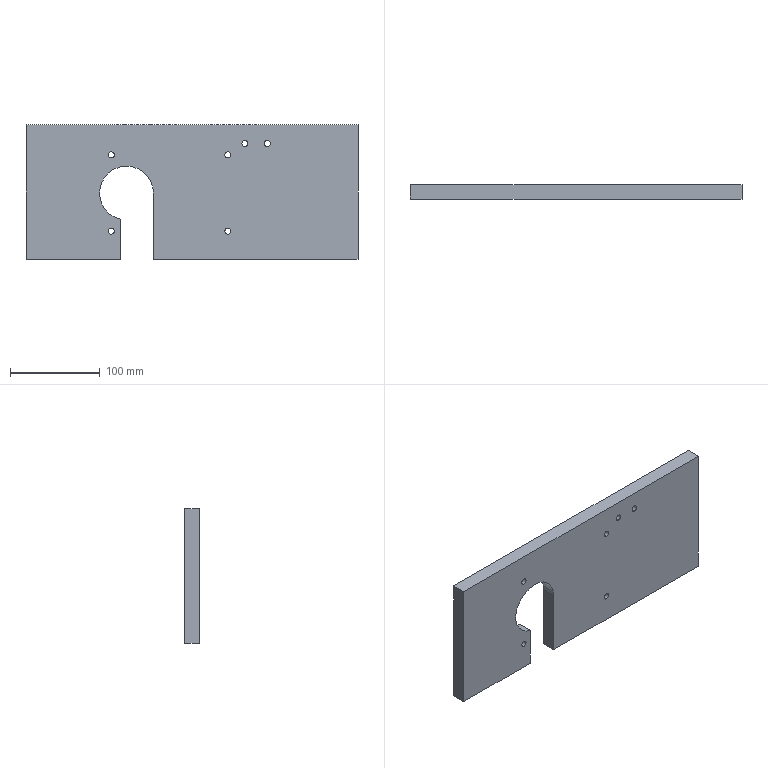Part | SolidWorks | features BaseBody 1 | 1 solid | 23 faces | box 370 x 16 x 150 mm | volume 810224 mm3 | cylinder 14 | plane 9 | commonest cylinder face diameters 6.8 x12 60 x2
STEP:
#1=CARTESIAN_POINT('',(-73.,0.,28.8));
#2=VERTEX_POINT('',#1);
#3=CARTESIAN_POINT('',(-43.,0.,-1.2));
#4=VERTEX_POINT('',#3);
#5=CARTESIAN_POINT('',(-73.,0.,-1.2));
#6=DIRECTION('',(0.,1.,0.));
#7=DIRECTION('',(0.,0.,1.));
#8=AXIS2_PLACEMENT_3D('',#5,#6,#7);
#9=CIRCLE('',#8,30.);
#10=EDGE_CURVE('',#2,#4,#9,.T.);
#11=ORIENTED_EDGE('',*,*,#10,.F.);
#12=CARTESIAN_POINT('',(-73.,16.,28.8));
#13=VERTEX_POINT('',#12);
#14=CARTESIAN_POINT('',(-73.,0.,28.8));
#15=DIRECTION('',(0.,1.,0.));
#16=VECTOR('',#15,1000.);
#17=LINE('',#14,#16);
#18=EDGE_CURVE('',#2,#13,#17,.T.);
#19=ORIENTED_EDGE('',*,*,#18,.T.);
#20=CARTESIAN_POINT('',(-43.,16.,-1.2));
#21=VERTEX_POINT('',#20);
#22=CARTESIAN_POINT('',(-73.,16.,-1.2));
#23=DIRECTION('',(0.,1.,0.));
#24=DIRECTION('',(0.,0.,1.));
#25=AXIS2_PLACEMENT_3D('',#22,#23,#24);
#26=CIRCLE('',#25,30.);
#27=EDGE_CURVE('',#13,#21,#26,.T.);
#28=ORIENTED_EDGE('',*,*,#27,.T.);
#29=CARTESIAN_POINT('',(-43.,0.,-1.2));
#30=DIRECTION('',(0.,-1.,0.));
#31=VECTOR('',#30,1000.);
#32=LINE('',#29,#31);
#33=EDGE_CURVE('',#21,#4,#32,.T.);
#34=ORIENTED_EDGE('',*,*,#33,.T.);
#35=EDGE_LOOP('',(#11,#19,#28,#34));
#36=FACE_OUTER_BOUND('',#35,.T.);
#37=CARTESIAN_POINT('',(-73.,0.,-1.2));
#38=DIRECTION('',(0.,1.,0.));
#39=DIRECTION('',(0.,0.,1.));
#40=AXIS2_PLACEMENT_3D('',#37,#38,#39);
#41=CYLINDRICAL_SURFACE('',#40,30.);
#42=ADVANCED_FACE('',(#36),#41,.F.);
#43=CARTESIAN_POINT('',(-90.,0.,37.9));
#44=VERTEX_POINT('',#43);
#45=CARTESIAN_POINT('',(-90.,0.,44.7));
#46=VERTEX_POINT('',#45);
#47=CARTESIAN_POINT('',(-90.,0.,41.3));
#48=DIRECTION('',(0.,1.,0.));
#49=DIRECTION('',(0.,0.,1.));
#50=AXIS2_PLACEMENT_3D('',#47,#48,#49);
#51=CIRCLE('',#50,3.4);
#52=EDGE_CURVE('',#44,#46,#51,.T.);
#53=ORIENTED_EDGE('',*,*,#52,.F.);
#54=CARTESIAN_POINT('',(-90.,16.,37.9));
#55=VERTEX_POINT('',#54);
#56=CARTESIAN_POINT('',(-90.,16.,37.9));
#57=DIRECTION('',(0.,1.,0.));
#58=VECTOR('',#57,1000.);
#59=LINE('',#56,#58);
#60=EDGE_CURVE('',#44,#55,#59,.T.);
#61=ORIENTED_EDGE('',*,*,#60,.T.);
#62=CARTESIAN_POINT('',(-90.,16.,44.7));
#63=VERTEX_POINT('',#62);
#64=CARTESIAN_POINT('',(-90.,16.,41.3));
#65=DIRECTION('',(0.,1.,0.));
#66=DIRECTION('',(0.,0.,1.));
#67=AXIS2_PLACEMENT_3D('',#64,#65,#66);
#68=CIRCLE('',#67,3.4);
#69=EDGE_CURVE('',#55,#63,#68,.T.);
#70=ORIENTED_EDGE('',*,*,#69,.T.);
#71=CARTESIAN_POINT('',(-90.,16.,44.7));
#72=DIRECTION('',(0.,1.,0.));
#73=VECTOR('',#72,1000.);
#74=LINE('',#71,#73);
#75=EDGE_CURVE('',#46,#63,#74,.T.);
#76=ORIENTED_EDGE('',*,*,#75,.F.);
#77=EDGE_LOOP('',(#53,#61,#70,#76));
#78=FACE_OUTER_BOUND('',#77,.T.);
#79=CARTESIAN_POINT('',(-90.,16.,41.3));
#80=DIRECTION('',(0.,1.,0.));
#81=DIRECTION('',(0.,0.,1.));
#82=AXIS2_PLACEMENT_3D('',#79,#80,#81);
#83=CYLINDRICAL_SURFACE('',#82,3.4);
#84=ADVANCED_FACE('',(#78),#83,.F.);
#85=CARTESIAN_POINT('',(-90.,0.,-47.1));
#86=VERTEX_POINT('',#85);
#87=CARTESIAN_POINT('',(-90.,0.,-40.3));
#88=VERTEX_POINT('',#87);
#89=CARTESIAN_POINT('',(-90.,0.,-43.7));
#90=DIRECTION('',(0.,1.,0.));
#91=DIRECTION('',(0.,0.,1.));
#92=AXIS2_PLACEMENT_3D('',#89,#90,#91);
#93=CIRCLE('',#92,3.4);
#94=EDGE_CURVE('',#86,#88,#93,.T.);
#95=ORIENTED_EDGE('',*,*,#94,.F.);
#96=CARTESIAN_POINT('',(-90.,16.,-47.1));
#97=VERTEX_POINT('',#96);
#98=CARTESIAN_POINT('',(-90.,16.,-47.1));
#99=DIRECTION('',(0.,1.,0.));
#100=VECTOR('',#99,1000.);
#101=LINE('',#98,#100);
#102=EDGE_CURVE('',#86,#97,#101,.T.);
#103=ORIENTED_EDGE('',*,*,#102,.T.);
#104=CARTESIAN_POINT('',(-90.,16.,-40.3));
#105=VERTEX_POINT('',#104);
#106=CARTESIAN_POINT('',(-90.,16.,-43.7));
#107=DIRECTION('',(0.,1.,0.));
#108=DIRECTION('',(0.,0.,1.));
#109=AXIS2_PLACEMENT_3D('',#106,#107,#108);
#110=CIRCLE('',#109,3.4);
#111=EDGE_CURVE('',#97,#105,#110,.T.);
#112=ORIENTED_EDGE('',*,*,#111,.T.);
#113=CARTESIAN_POINT('',(-90.,16.,-40.3));
#114=DIRECTION('',(0.,1.,0.));
#115=VECTOR('',#114,1000.);
#116=LINE('',#113,#115);
#117=EDGE_CURVE('',#88,#105,#116,.T.);
#118=ORIENTED_EDGE('',*,*,#117,.F.);
#119=EDGE_LOOP('',(#95,#103,#112,#118));
#120=FACE_OUTER_BOUND('',#119,.T.);
#121=CARTESIAN_POINT('',(-90.,16.,-43.7));
#122=DIRECTION('',(0.,1.,0.));
#123=DIRECTION('',(0.,0.,1.));
#124=AXIS2_PLACEMENT_3D('',#121,#122,#123);
#125=CYLINDRICAL_SURFACE('',#124,3.4);
#126=ADVANCED_FACE('',(#120),#125,.F.);
#127=CARTESIAN_POINT('',(40.,0.,-47.1));
#128=VERTEX_POINT('',#127);
#129=CARTESIAN_POINT('',(40.,0.,-40.3));
#130=VERTEX_POINT('',#129);
#131=CARTESIAN_POINT('',(40.,0.,-43.7));
#132=DIRECTION('',(0.,1.,0.));
#133=DIRECTION('',(0.,0.,1.));
#134=AXIS2_PLACEMENT_3D('',#131,#132,#133);
#135=CIRCLE('',#134,3.4);
#136=EDGE_CURVE('',#128,#130,#135,.T.);
#137=ORIENTED_EDGE('',*,*,#136,.F.);
#138=CARTESIAN_POINT('',(40.,16.,-47.1));
#139=VERTEX_POINT('',#138);
#140=CARTESIAN_POINT('',(40.,16.,-47.1));
#141=DIRECTION('',(0.,1.,0.));
#142=VECTOR('',#141,1000.);
#143=LINE('',#140,#142);
#144=EDGE_CURVE('',#128,#139,#143,.T.);
#145=ORIENTED_EDGE('',*,*,#144,.T.);
#146=CARTESIAN_POINT('',(40.,16.,-40.3));
#147=VERTEX_POINT('',#146);
#148=CARTESIAN_POINT('',(40.,16.,-43.7));
#149=DIRECTION('',(0.,1.,0.));
#150=DIRECTION('',(0.,0.,1.));
#151=AXIS2_PLACEMENT_3D('',#148,#149,#150);
#152=CIRCLE('',#151,3.4);
#153=EDGE_CURVE('',#139,#147,#152,.T.);
#154=ORIENTED_EDGE('',*,*,#153,.T.);
#155=CARTESIAN_POINT('',(40.,16.,-40.3));
#156=DIRECTION('',(0.,1.,0.));
#157=VECTOR('',#156,1000.);
#158=LINE('',#155,#157);
#159=EDGE_CURVE('',#130,#147,#158,.T.);
#160=ORIENTED_EDGE('',*,*,#159,.F.);
#161=EDGE_LOOP('',(#137,#145,#154,#160));
#162=FACE_OUTER_BOUND('',#161,.T.);
#163=CARTESIAN_POINT('',(40.,16.,-43.7));
#164=DIRECTION('',(0.,1.,0.));
#165=DIRECTION('',(0.,0.,1.));
#166=AXIS2_PLACEMENT_3D('',#163,#164,#165);
#167=CYLINDRICAL_SURFACE('',#166,3.4);
#168=ADVANCED_FACE('',(#162),#167,.F.);
#169=CARTESIAN_POINT('',(40.,0.,37.9));
#170=VERTEX_POINT('',#169);
#171=CARTESIAN_POINT('',(40.,0.,44.7));
#172=VERTEX_POINT('',#171);
#173=CARTESIAN_POINT('',(40.,0.,41.3));
#174=DIRECTION('',(0.,1.,0.));
#175=DIRECTION('',(0.,0.,1.));
#176=AXIS2_PLACEMENT_3D('',#173,#174,#175);
#177=CIRCLE('',#176,3.4);
#178=EDGE_CURVE('',#170,#172,#177,.T.);
#179=ORIENTED_EDGE('',*,*,#178,.F.);
#180=CARTESIAN_POINT('',(40.,16.,37.9));
#181=VERTEX_POINT('',#180);
#182=CARTESIAN_POINT('',(40.,16.,37.9));
#183=DIRECTION('',(0.,1.,0.));
#184=VECTOR('',#183,1000.);
#185=LINE('',#182,#184);
#186=EDGE_CURVE('',#170,#181,#185,.T.);
#187=ORIENTED_EDGE('',*,*,#186,.T.);
#188=CARTESIAN_POINT('',(40.,16.,44.7));
#189=VERTEX_POINT('',#188);
#190=CARTESIAN_POINT('',(40.,16.,41.3));
#191=DIRECTION('',(0.,1.,0.));
#192=DIRECTION('',(0.,0.,1.));
#193=AXIS2_PLACEMENT_3D('',#190,#191,#192);
#194=CIRCLE('',#193,3.4);
#195=EDGE_CURVE('',#181,#189,#194,.T.);
#196=ORIENTED_EDGE('',*,*,#195,.T.);
#197=CARTESIAN_POINT('',(40.,16.,44.7));
#198=DIRECTION('',(0.,1.,0.));
#199=VECTOR('',#198,1000.);
#200=LINE('',#197,#199);
#201=EDGE_CURVE('',#172,#189,#200,.T.);
#202=ORIENTED_EDGE('',*,*,#201,.F.);
#203=EDGE_LOOP('',(#179,#187,#196,#202));
#204=FACE_OUTER_BOUND('',#203,.T.);
#205=CARTESIAN_POINT('',(40.,16.,41.3));
#206=DIRECTION('',(0.,1.,0.));
#207=DIRECTION('',(0.,0.,1.));
#208=AXIS2_PLACEMENT_3D('',#205,#206,#207);
#209=CYLINDRICAL_SURFACE('',#208,3.4);
#210=ADVANCED_FACE('',(#204),#209,.F.);
#211=CARTESIAN_POINT('',(58.921,0.,50.6));
#212=VERTEX_POINT('',#211);
#213=CARTESIAN_POINT('',(58.921,0.,57.4));
#214=VERTEX_POINT('',#213);
#215=CARTESIAN_POINT('',(58.921,0.,54.));
#216=DIRECTION('',(0.,1.,0.));
#217=DIRECTION('',(0.,0.,1.));
#218=AXIS2_PLACEMENT_3D('',#215,#216,#217);
#219=CIRCLE('',#218,3.4);
#220=EDGE_CURVE('',#212,#214,#219,.T.);
#221=ORIENTED_EDGE('',*,*,#220,.F.);
#222=CARTESIAN_POINT('',(58.921,16.,50.6));
#223=VERTEX_POINT('',#222);
#224=CARTESIAN_POINT('',(58.921,16.,50.6));
#225=DIRECTION('',(0.,1.,0.));
#226=VECTOR('',#225,1000.);
#227=LINE('',#224,#226);
#228=EDGE_CURVE('',#212,#223,#227,.T.);
#229=ORIENTED_EDGE('',*,*,#228,.T.);
#230=CARTESIAN_POINT('',(58.921,16.,57.4));
#231=VERTEX_POINT('',#230);
#232=CARTESIAN_POINT('',(58.921,16.,54.));
#233=DIRECTION('',(0.,1.,0.));
#234=DIRECTION('',(0.,0.,1.));
#235=AXIS2_PLACEMENT_3D('',#232,#233,#234);
#236=CIRCLE('',#235,3.4);
#237=EDGE_CURVE('',#223,#231,#236,.T.);
#238=ORIENTED_EDGE('',*,*,#237,.T.);
#239=CARTESIAN_POINT('',(58.921,16.,57.4));
#240=DIRECTION('',(0.,1.,0.));
#241=VECTOR('',#240,1000.);
#242=LINE('',#239,#241);
#243=EDGE_CURVE('',#214,#231,#242,.T.);
#244=ORIENTED_EDGE('',*,*,#243,.F.);
#245=EDGE_LOOP('',(#221,#229,#238,#244));
#246=FACE_OUTER_BOUND('',#245,.T.);
#247=CARTESIAN_POINT('',(58.921,16.,54.));
#248=DIRECTION('',(0.,1.,0.));
#249=DIRECTION('',(0.,0.,1.));
#250=AXIS2_PLACEMENT_3D('',#247,#248,#249);
#251=CYLINDRICAL_SURFACE('',#250,3.4);
#252=ADVANCED_FACE('',(#246),#251,.F.);
#253=CARTESIAN_POINT('',(83.921,0.,50.6));
#254=VERTEX_POINT('',#253);
#255=CARTESIAN_POINT('',(83.921,0.,57.4));
#256=VERTEX_POINT('',#255);
#257=CARTESIAN_POINT('',(83.921,0.,54.));
#258=DIRECTION('',(0.,1.,0.));
#259=DIRECTION('',(0.,0.,1.));
#260=AXIS2_PLACEMENT_3D('',#257,#258,#259);
#261=CIRCLE('',#260,3.4);
#262=EDGE_CURVE('',#254,#256,#261,.T.);
#263=ORIENTED_EDGE('',*,*,#262,.F.);
#264=CARTESIAN_POINT('',(83.921,16.,50.6));
#265=VERTEX_POINT('',#264);
#266=CARTESIAN_POINT('',(83.921,16.,50.6));
#267=DIRECTION('',(0.,1.,0.));
#268=VECTOR('',#267,1000.);
#269=LINE('',#266,#268);
#270=EDGE_CURVE('',#254,#265,#269,.T.);
#271=ORIENTED_EDGE('',*,*,#270,.T.);
#272=CARTESIAN_POINT('',(83.921,16.,57.4));
#273=VERTEX_POINT('',#272);
#274=CARTESIAN_POINT('',(83.921,16.,54.));
#275=DIRECTION('',(0.,1.,0.));
#276=DIRECTION('',(0.,0.,1.));
#277=AXIS2_PLACEMENT_3D('',#274,#275,#276);
#278=CIRCLE('',#277,3.4);
#279=EDGE_CURVE('',#265,#273,#278,.T.);
#280=ORIENTED_EDGE('',*,*,#279,.T.);
#281=CARTESIAN_POINT('',(83.921,16.,57.4));
#282=DIRECTION('',(0.,1.,0.));
#283=VECTOR('',#282,1000.);
#284=LINE('',#281,#283);
#285=EDGE_CURVE('',#256,#273,#284,.T.);
#286=ORIENTED_EDGE('',*,*,#285,.F.);
#287=EDGE_LOOP('',(#263,#271,#280,#286));
#288=FACE_OUTER_BOUND('',#287,.T.);
#289=CARTESIAN_POINT('',(83.921,16.,54.));
#290=DIRECTION('',(0.,1.,0.));
#291=DIRECTION('',(0.,0.,1.));
#292=AXIS2_PLACEMENT_3D('',#289,#290,#291);
#293=CYLINDRICAL_SURFACE('',#292,3.4);
#294=ADVANCED_FACE('',(#288),#293,.F.);
#295=CARTESIAN_POINT('',(-80.,16.,-75.));
#296=VERTEX_POINT('',#295);
#297=CARTESIAN_POINT('',(-80.,16.,-30.372));
#298=VERTEX_POINT('',#297);
#299=CARTESIAN_POINT('',(-80.,16.,0.));
#300=DIRECTION('',(0.,0.,1.));
#301=VECTOR('',#300,1000.);
#302=LINE('',#299,#301);
#303=EDGE_CURVE('',#296,#298,#302,.T.);
#304=ORIENTED_EDGE('',*,*,#303,.F.);
#305=CARTESIAN_POINT('',(-185.,16.,-75.));
#306=VERTEX_POINT('',#305);
#307=CARTESIAN_POINT('',(0.,16.,-75.));
#308=DIRECTION('',(1.,0.,0.));
#309=VECTOR('',#308,1000.);
#310=LINE('',#307,#309);
#311=EDGE_CURVE('',#306,#296,#310,.T.);
#312=ORIENTED_EDGE('',*,*,#311,.F.);
#313=CARTESIAN_POINT('',(-185.,16.,75.));
#314=VERTEX_POINT('',#313);
#315=CARTESIAN_POINT('',(-185.,16.,0.));
#316=DIRECTION('',(0.,0.,-1.));
#317=VECTOR('',#316,1000.);
#318=LINE('',#315,#317);
#319=EDGE_CURVE('',#314,#306,#318,.T.);
#320=ORIENTED_EDGE('',*,*,#319,.F.);
#321=CARTESIAN_POINT('',(185.,16.,75.));
#322=VERTEX_POINT('',#321);
#323=CARTESIAN_POINT('',(0.,16.,75.));
#324=DIRECTION('',(-1.,0.,0.));
#325=VECTOR('',#324,1000.);
#326=LINE('',#323,#325);
#327=EDGE_CURVE('',#322,#314,#326,.T.);
#328=ORIENTED_EDGE('',*,*,#327,.F.);
#329=CARTESIAN_POINT('',(185.,16.,-75.));
#330=VERTEX_POINT('',#329);
#331=CARTESIAN_POINT('',(185.,16.,0.));
#332=DIRECTION('',(0.,0.,1.));
#333=VECTOR('',#332,1000.);
#334=LINE('',#331,#333);
#335=EDGE_CURVE('',#330,#322,#334,.T.);
#336=ORIENTED_EDGE('',*,*,#335,.F.);
#337=CARTESIAN_POINT('',(-43.,16.,-75.));
#338=VERTEX_POINT('',#337);
#339=CARTESIAN_POINT('',(0.,16.,-75.));
#340=DIRECTION('',(1.,0.,0.));
#341=VECTOR('',#340,1000.);
#342=LINE('',#339,#341);
#343=EDGE_CURVE('',#338,#330,#342,.T.);
#344=ORIENTED_EDGE('',*,*,#343,.F.);
#345=CARTESIAN_POINT('',(-43.,16.,0.));
#346=DIRECTION('',(0.,0.,-1.));
#347=VECTOR('',#346,1000.);
#348=LINE('',#345,#347);
#349=EDGE_CURVE('',#21,#338,#348,.T.);
#350=ORIENTED_EDGE('',*,*,#349,.F.);
#351=ORIENTED_EDGE('',*,*,#27,.F.);
#352=CARTESIAN_POINT('',(-73.,16.,-1.2));
#353=DIRECTION('',(0.,1.,0.));
#354=DIRECTION('',(0.,0.,1.));
#355=AXIS2_PLACEMENT_3D('',#352,#353,#354);
#356=CIRCLE('',#355,30.);
#357=EDGE_CURVE('',#298,#13,#356,.T.);
#358=ORIENTED_EDGE('',*,*,#357,.F.);
#359=EDGE_LOOP('',(#304,#312,#320,#328,#336,#344,#350,#351,#358));
#360=FACE_OUTER_BOUND('',#359,.T.);
#361=CARTESIAN_POINT('',(-90.,16.,41.3));
#362=DIRECTION('',(0.,1.,0.));
#363=DIRECTION('',(0.,0.,1.));
#364=AXIS2_PLACEMENT_3D('',#361,#362,#363);
#365=CIRCLE('',#364,3.4);
#366=EDGE_CURVE('',#63,#55,#365,.T.);
#367=ORIENTED_EDGE('',*,*,#366,.F.);
#368=ORIENTED_EDGE('',*,*,#69,.F.);
#369=EDGE_LOOP('',(#367,#368));
#370=FACE_BOUND('',#369,.T.);
#371=CARTESIAN_POINT('',(-90.,16.,-43.7));
#372=DIRECTION('',(0.,1.,0.));
#373=DIRECTION('',(0.,0.,1.));
#374=AXIS2_PLACEMENT_3D('',#371,#372,#373);
#375=CIRCLE('',#374,3.4);
#376=EDGE_CURVE('',#105,#97,#375,.T.);
#377=ORIENTED_EDGE('',*,*,#376,.F.);
#378=ORIENTED_EDGE('',*,*,#111,.F.);
#379=EDGE_LOOP('',(#377,#378));
#380=FACE_BOUND('',#379,.T.);
#381=CARTESIAN_POINT('',(40.,16.,-43.7));
#382=DIRECTION('',(0.,1.,0.));
#383=DIRECTION('',(0.,0.,1.));
#384=AXIS2_PLACEMENT_3D('',#381,#382,#383);
#385=CIRCLE('',#384,3.4);
#386=EDGE_CURVE('',#147,#139,#385,.T.);
#387=ORIENTED_EDGE('',*,*,#386,.F.);
#388=ORIENTED_EDGE('',*,*,#153,.F.);
#389=EDGE_LOOP('',(#387,#388));
#390=FACE_BOUND('',#389,.T.);
#391=CARTESIAN_POINT('',(40.,16.,41.3));
#392=DIRECTION('',(0.,1.,0.));
#393=DIRECTION('',(0.,0.,1.));
#394=AXIS2_PLACEMENT_3D('',#391,#392,#393);
#395=CIRCLE('',#394,3.4);
#396=EDGE_CURVE('',#189,#181,#395,.T.);
#397=ORIENTED_EDGE('',*,*,#396,.F.);
#398=ORIENTED_EDGE('',*,*,#195,.F.);
#399=EDGE_LOOP('',(#397,#398));
#400=FACE_BOUND('',#399,.T.);
#401=CARTESIAN_POINT('',(58.921,16.,54.));
#402=DIRECTION('',(0.,1.,0.));
#403=DIRECTION('',(0.,0.,1.));
#404=AXIS2_PLACEMENT_3D('',#401,#402,#403);
#405=CIRCLE('',#404,3.4);
#406=EDGE_CURVE('',#231,#223,#405,.T.);
#407=ORIENTED_EDGE('',*,*,#406,.F.);
#408=ORIENTED_EDGE('',*,*,#237,.F.);
#409=EDGE_LOOP('',(#407,#408));
#410=FACE_BOUND('',#409,.T.);
#411=CARTESIAN_POINT('',(83.921,16.,54.));
#412=DIRECTION('',(0.,1.,0.));
#413=DIRECTION('',(0.,0.,1.));
#414=AXIS2_PLACEMENT_3D('',#411,#412,#413);
#415=CIRCLE('',#414,3.4);
#416=EDGE_CURVE('',#273,#265,#415,.T.);
#417=ORIENTED_EDGE('',*,*,#416,.F.);
#418=ORIENTED_EDGE('',*,*,#279,.F.);
#419=EDGE_LOOP('',(#417,#418));
#420=FACE_BOUND('',#419,.T.);
#421=CARTESIAN_POINT('',(0.,16.,0.));
#422=DIRECTION('',(0.,-1.,0.));
#423=DIRECTION('',(0.,0.,-1.));
#424=AXIS2_PLACEMENT_3D('',#421,#422,#423);
#425=PLANE('',#424);
#426=ADVANCED_FACE('',(#360,#370,#380,#390,#400,#410,#420),#425,.F.);
#427=ORIENTED_EDGE('',*,*,#18,.F.);
#428=CARTESIAN_POINT('',(-80.,0.,-30.372));
#429=VERTEX_POINT('',#428);
#430=CARTESIAN_POINT('',(-73.,0.,-1.2));
#431=DIRECTION('',(0.,1.,0.));
#432=DIRECTION('',(0.,0.,1.));
#433=AXIS2_PLACEMENT_3D('',#430,#431,#432);
#434=CIRCLE('',#433,30.);
#435=EDGE_CURVE('',#429,#2,#434,.T.);
#436=ORIENTED_EDGE('',*,*,#435,.F.);
#437=CARTESIAN_POINT('',(-80.,0.,-30.372));
#438=DIRECTION('',(0.,-1.,0.));
#439=VECTOR('',#438,1000.);
#440=LINE('',#437,#439);
#441=EDGE_CURVE('',#298,#429,#440,.T.);
#442=ORIENTED_EDGE('',*,*,#441,.F.);
#443=ORIENTED_EDGE('',*,*,#357,.T.);
#444=EDGE_LOOP('',(#427,#436,#442,#443));
#445=FACE_OUTER_BOUND('',#444,.T.);
#446=CARTESIAN_POINT('',(-73.,0.,-1.2));
#447=DIRECTION('',(0.,1.,0.));
#448=DIRECTION('',(0.,0.,1.));
#449=AXIS2_PLACEMENT_3D('',#446,#447,#448);
#450=CYLINDRICAL_SURFACE('',#449,30.);
#451=ADVANCED_FACE('',(#445),#450,.F.);
#452=ORIENTED_EDGE('',*,*,#441,.T.);
#453=CARTESIAN_POINT('',(-80.,0.,-75.));
#454=VERTEX_POINT('',#453);
#455=CARTESIAN_POINT('',(-80.,0.,-99.691));
#456=DIRECTION('',(0.,0.,1.));
#457=VECTOR('',#456,1000.);
#458=LINE('',#455,#457);
#459=EDGE_CURVE('',#454,#429,#458,.T.);
#460=ORIENTED_EDGE('',*,*,#459,.F.);
#461=CARTESIAN_POINT('',(-80.,0.,-75.));
#462=DIRECTION('',(0.,-1.,0.));
#463=VECTOR('',#462,1000.);
#464=LINE('',#461,#463);
#465=EDGE_CURVE('',#296,#454,#464,.T.);
#466=ORIENTED_EDGE('',*,*,#465,.F.);
#467=ORIENTED_EDGE('',*,*,#303,.T.);
#468=EDGE_LOOP('',(#452,#460,#466,#467));
#469=FACE_OUTER_BOUND('',#468,.T.);
#470=CARTESIAN_POINT('',(-80.,0.,-99.691));
#471=DIRECTION('',(-1.,0.,0.));
#472=DIRECTION('',(0.,0.,1.));
#473=AXIS2_PLACEMENT_3D('',#470,#471,#472);
#474=PLANE('',#473);
#475=ADVANCED_FACE('',(#469),#474,.F.);
#476=ORIENTED_EDGE('',*,*,#465,.T.);
#477=CARTESIAN_POINT('',(-185.,0.,-75.));
#478=VERTEX_POINT('',#477);
#479=CARTESIAN_POINT('',(-185.,0.,-75.));
#480=DIRECTION('',(1.,0.,0.));
#481=VECTOR('',#480,1000.);
#482=LINE('',#479,#481);
#483=EDGE_CURVE('',#478,#454,#482,.T.);
#484=ORIENTED_EDGE('',*,*,#483,.F.);
#485=CARTESIAN_POINT('',(-185.,16.,-75.));
#486=DIRECTION('',(0.,-1.,0.));
#487=VECTOR('',#486,1000.);
#488=LINE('',#485,#487);
#489=EDGE_CURVE('',#306,#478,#488,.T.);
#490=ORIENTED_EDGE('',*,*,#489,.F.);
#491=ORIENTED_EDGE('',*,*,#311,.T.);
#492=EDGE_LOOP('',(#476,#484,#490,#491));
#493=FACE_OUTER_BOUND('',#492,.T.);
#494=CARTESIAN_POINT('',(-185.,16.,-75.));
#495=DIRECTION('',(0.,0.,1.));
#496=DIRECTION('',(1.,0.,0.));
#497=AXIS2_PLACEMENT_3D('',#494,#495,#496);
#498=PLANE('',#497);
#499=ADVANCED_FACE('',(#493),#498,.F.);
#500=CARTESIAN_POINT('',(-185.,0.,75.));
#501=VERTEX_POINT('',#500);
#502=CARTESIAN_POINT('',(-185.,16.,75.));
#503=DIRECTION('',(0.,-1.,0.));
#504=VECTOR('',#503,1000.);
#505=LINE('',#502,#504);
#506=EDGE_CURVE('',#314,#501,#505,.T.);
#507=ORIENTED_EDGE('',*,*,#506,.F.);
#508=ORIENTED_EDGE('',*,*,#319,.T.);
#509=ORIENTED_EDGE('',*,*,#489,.T.);
#510=CARTESIAN_POINT('',(-185.,0.,75.));
#511=DIRECTION('',(0.,0.,-1.));
#512=VECTOR('',#511,1000.);
#513=LINE('',#510,#512);
#514=EDGE_CURVE('',#501,#478,#513,.T.);
#515=ORIENTED_EDGE('',*,*,#514,.F.);
#516=EDGE_LOOP('',(#507,#508,#509,#515));
#517=FACE_OUTER_BOUND('',#516,.T.);
#518=CARTESIAN_POINT('',(-185.,16.,75.));
#519=DIRECTION('',(1.,0.,0.));
#520=DIRECTION('',(0.,0.,-1.));
#521=AXIS2_PLACEMENT_3D('',#518,#519,#520);
#522=PLANE('',#521);
#523=ADVANCED_FACE('',(#517),#522,.F.);
#524=CARTESIAN_POINT('',(185.,0.,75.));
#525=VERTEX_POINT('',#524);
#526=CARTESIAN_POINT('',(185.,16.,75.));
#527=DIRECTION('',(0.,-1.,0.));
#528=VECTOR('',#527,1000.);
#529=LINE('',#526,#528);
#530=EDGE_CURVE('',#322,#525,#529,.T.);
#531=ORIENTED_EDGE('',*,*,#530,.F.);
#532=ORIENTED_EDGE('',*,*,#327,.T.);
#533=ORIENTED_EDGE('',*,*,#506,.T.);
#534=CARTESIAN_POINT('',(-185.,0.,75.));
#535=DIRECTION('',(-1.,0.,0.));
#536=VECTOR('',#535,1000.);
#537=LINE('',#534,#536);
#538=EDGE_CURVE('',#525,#501,#537,.T.);
#539=ORIENTED_EDGE('',*,*,#538,.F.);
#540=EDGE_LOOP('',(#531,#532,#533,#539));
#541=FACE_OUTER_BOUND('',#540,.T.);
#542=CARTESIAN_POINT('',(-185.,16.,75.));
#543=DIRECTION('',(0.,0.,-1.));
#544=DIRECTION('',(-1.,0.,0.));
#545=AXIS2_PLACEMENT_3D('',#542,#543,#544);
#546=PLANE('',#545);
#547=ADVANCED_FACE('',(#541),#546,.F.);
#548=CARTESIAN_POINT('',(185.,0.,-75.));
#549=VERTEX_POINT('',#548);
#550=CARTESIAN_POINT('',(185.,16.,-75.));
#551=DIRECTION('',(0.,-1.,0.));
#552=VECTOR('',#551,1000.);
#553=LINE('',#550,#552);
#554=EDGE_CURVE('',#330,#549,#553,.T.);
#555=ORIENTED_EDGE('',*,*,#554,.F.);
#556=ORIENTED_EDGE('',*,*,#335,.T.);
#557=ORIENTED_EDGE('',*,*,#530,.T.);
#558=CARTESIAN_POINT('',(185.,0.,75.));
#559=DIRECTION('',(0.,0.,1.));
#560=VECTOR('',#559,1000.);
#561=LINE('',#558,#560);
#562=EDGE_CURVE('',#549,#525,#561,.T.);
#563=ORIENTED_EDGE('',*,*,#562,.F.);
#564=EDGE_LOOP('',(#555,#556,#557,#563));
#565=FACE_OUTER_BOUND('',#564,.T.);
#566=CARTESIAN_POINT('',(185.,16.,75.));
#567=DIRECTION('',(-1.,0.,0.));
#568=DIRECTION('',(0.,0.,1.));
#569=AXIS2_PLACEMENT_3D('',#566,#567,#568);
#570=PLANE('',#569);
#571=ADVANCED_FACE('',(#565),#570,.F.);
#572=CARTESIAN_POINT('',(-43.,0.,-75.));
#573=VERTEX_POINT('',#572);
#574=CARTESIAN_POINT('',(-43.,16.,-75.));
#575=DIRECTION('',(0.,-1.,0.));
#576=VECTOR('',#575,1000.);
#577=LINE('',#574,#576);
#578=EDGE_CURVE('',#338,#573,#577,.T.);
#579=ORIENTED_EDGE('',*,*,#578,.F.);
#580=ORIENTED_EDGE('',*,*,#343,.T.);
#581=ORIENTED_EDGE('',*,*,#554,.T.);
#582=CARTESIAN_POINT('',(-185.,0.,-75.));
#583=DIRECTION('',(1.,0.,0.));
#584=VECTOR('',#583,1000.);
#585=LINE('',#582,#584);
#586=EDGE_CURVE('',#573,#549,#585,.T.);
#587=ORIENTED_EDGE('',*,*,#586,.F.);
#588=EDGE_LOOP('',(#579,#580,#581,#587));
#589=FACE_OUTER_BOUND('',#588,.T.);
#590=CARTESIAN_POINT('',(-185.,16.,-75.));
#591=DIRECTION('',(0.,0.,1.));
#592=DIRECTION('',(1.,0.,0.));
#593=AXIS2_PLACEMENT_3D('',#590,#591,#592);
#594=PLANE('',#593);
#595=ADVANCED_FACE('',(#589),#594,.F.);
#596=ORIENTED_EDGE('',*,*,#33,.F.);
#597=ORIENTED_EDGE('',*,*,#349,.T.);
#598=ORIENTED_EDGE('',*,*,#578,.T.);
#599=CARTESIAN_POINT('',(-43.,0.,-1.2));
#600=DIRECTION('',(0.,0.,-1.));
#601=VECTOR('',#600,1000.);
#602=LINE('',#599,#601);
#603=EDGE_CURVE('',#4,#573,#602,.T.);
#604=ORIENTED_EDGE('',*,*,#603,.F.);
#605=EDGE_LOOP('',(#596,#597,#598,#604));
#606=FACE_OUTER_BOUND('',#605,.T.);
#607=CARTESIAN_POINT('',(-43.,0.,-1.2));
#608=DIRECTION('',(1.,0.,0.));
#609=DIRECTION('',(0.,0.,-1.));
#610=AXIS2_PLACEMENT_3D('',#607,#608,#609);
#611=PLANE('',#610);
#612=ADVANCED_FACE('',(#606),#611,.F.);
#613=ORIENTED_EDGE('',*,*,#60,.F.);
#614=CARTESIAN_POINT('',(-90.,0.,41.3));
#615=DIRECTION('',(0.,1.,0.));
#616=DIRECTION('',(0.,0.,1.));
#617=AXIS2_PLACEMENT_3D('',#614,#615,#616);
#618=CIRCLE('',#617,3.4);
#619=EDGE_CURVE('',#46,#44,#618,.T.);
#620=ORIENTED_EDGE('',*,*,#619,.F.);
#621=ORIENTED_EDGE('',*,*,#75,.T.);
#622=ORIENTED_EDGE('',*,*,#366,.T.);
#623=EDGE_LOOP('',(#613,#620,#621,#622));
#624=FACE_OUTER_BOUND('',#623,.T.);
#625=CARTESIAN_POINT('',(-90.,16.,41.3));
#626=DIRECTION('',(0.,1.,0.));
#627=DIRECTION('',(0.,0.,1.));
#628=AXIS2_PLACEMENT_3D('',#625,#626,#627);
#629=CYLINDRICAL_SURFACE('',#628,3.4);
#630=ADVANCED_FACE('',(#624),#629,.F.);
#631=ORIENTED_EDGE('',*,*,#102,.F.);
#632=CARTESIAN_POINT('',(-90.,0.,-43.7));
#633=DIRECTION('',(0.,1.,0.));
#634=DIRECTION('',(0.,0.,1.));
#635=AXIS2_PLACEMENT_3D('',#632,#633,#634);
#636=CIRCLE('',#635,3.4);
#637=EDGE_CURVE('',#88,#86,#636,.T.);
#638=ORIENTED_EDGE('',*,*,#637,.F.);
#639=ORIENTED_EDGE('',*,*,#117,.T.);
#640=ORIENTED_EDGE('',*,*,#376,.T.);
#641=EDGE_LOOP('',(#631,#638,#639,#640));
#642=FACE_OUTER_BOUND('',#641,.T.);
#643=CARTESIAN_POINT('',(-90.,16.,-43.7));
#644=DIRECTION('',(0.,1.,0.));
#645=DIRECTION('',(0.,0.,1.));
#646=AXIS2_PLACEMENT_3D('',#643,#644,#645);
#647=CYLINDRICAL_SURFACE('',#646,3.4);
#648=ADVANCED_FACE('',(#642),#647,.F.);
#649=ORIENTED_EDGE('',*,*,#144,.F.);
#650=CARTESIAN_POINT('',(40.,0.,-43.7));
#651=DIRECTION('',(0.,1.,0.));
#652=DIRECTION('',(0.,0.,1.));
#653=AXIS2_PLACEMENT_3D('',#650,#651,#652);
#654=CIRCLE('',#653,3.4);
#655=EDGE_CURVE('',#130,#128,#654,.T.);
#656=ORIENTED_EDGE('',*,*,#655,.F.);
#657=ORIENTED_EDGE('',*,*,#159,.T.);
#658=ORIENTED_EDGE('',*,*,#386,.T.);
#659=EDGE_LOOP('',(#649,#656,#657,#658));
#660=FACE_OUTER_BOUND('',#659,.T.);
#661=CARTESIAN_POINT('',(40.,16.,-43.7));
#662=DIRECTION('',(0.,1.,0.));
#663=DIRECTION('',(0.,0.,1.));
#664=AXIS2_PLACEMENT_3D('',#661,#662,#663);
#665=CYLINDRICAL_SURFACE('',#664,3.4);
#666=ADVANCED_FACE('',(#660),#665,.F.);
#667=ORIENTED_EDGE('',*,*,#186,.F.);
#668=CARTESIAN_POINT('',(40.,0.,41.3));
#669=DIRECTION('',(0.,1.,0.));
#670=DIRECTION('',(0.,0.,1.));
#671=AXIS2_PLACEMENT_3D('',#668,#669,#670);
#672=CIRCLE('',#671,3.4);
#673=EDGE_CURVE('',#172,#170,#672,.T.);
#674=ORIENTED_EDGE('',*,*,#673,.F.);
#675=ORIENTED_EDGE('',*,*,#201,.T.);
#676=ORIENTED_EDGE('',*,*,#396,.T.);
#677=EDGE_LOOP('',(#667,#674,#675,#676));
#678=FACE_OUTER_BOUND('',#677,.T.);
#679=CARTESIAN_POINT('',(40.,16.,41.3));
#680=DIRECTION('',(0.,1.,0.));
#681=DIRECTION('',(0.,0.,1.));
#682=AXIS2_PLACEMENT_3D('',#679,#680,#681);
#683=CYLINDRICAL_SURFACE('',#682,3.4);
#684=ADVANCED_FACE('',(#678),#683,.F.);
#685=ORIENTED_EDGE('',*,*,#228,.F.);
#686=CARTESIAN_POINT('',(58.921,0.,54.));
#687=DIRECTION('',(0.,1.,0.));
#688=DIRECTION('',(0.,0.,1.));
#689=AXIS2_PLACEMENT_3D('',#686,#687,#688);
#690=CIRCLE('',#689,3.4);
#691=EDGE_CURVE('',#214,#212,#690,.T.);
#692=ORIENTED_EDGE('',*,*,#691,.F.);
#693=ORIENTED_EDGE('',*,*,#243,.T.);
#694=ORIENTED_EDGE('',*,*,#406,.T.);
#695=EDGE_LOOP('',(#685,#692,#693,#694));
#696=FACE_OUTER_BOUND('',#695,.T.);
#697=CARTESIAN_POINT('',(58.921,16.,54.));
#698=DIRECTION('',(0.,1.,0.));
#699=DIRECTION('',(0.,0.,1.));
#700=AXIS2_PLACEMENT_3D('',#697,#698,#699);
#701=CYLINDRICAL_SURFACE('',#700,3.4);
#702=ADVANCED_FACE('',(#696),#701,.F.);
#703=ORIENTED_EDGE('',*,*,#270,.F.);
#704=CARTESIAN_POINT('',(83.921,0.,54.));
#705=DIRECTION('',(0.,1.,0.));
#706=DIRECTION('',(0.,0.,1.));
#707=AXIS2_PLACEMENT_3D('',#704,#705,#706);
#708=CIRCLE('',#707,3.4);
#709=EDGE_CURVE('',#256,#254,#708,.T.);
#710=ORIENTED_EDGE('',*,*,#709,.F.);
#711=ORIENTED_EDGE('',*,*,#285,.T.);
#712=ORIENTED_EDGE('',*,*,#416,.T.);
#713=EDGE_LOOP('',(#703,#710,#711,#712));
#714=FACE_OUTER_BOUND('',#713,.T.);
#715=CARTESIAN_POINT('',(83.921,16.,54.));
#716=DIRECTION('',(0.,1.,0.));
#717=DIRECTION('',(0.,0.,1.));
#718=AXIS2_PLACEMENT_3D('',#715,#716,#717);
#719=CYLINDRICAL_SURFACE('',#718,3.4);
#720=ADVANCED_FACE('',(#714),#719,.F.);
#721=ORIENTED_EDGE('',*,*,#514,.T.);
#722=ORIENTED_EDGE('',*,*,#483,.T.);
#723=ORIENTED_EDGE('',*,*,#459,.T.);
#724=ORIENTED_EDGE('',*,*,#435,.T.);
#725=ORIENTED_EDGE('',*,*,#10,.T.);
#726=ORIENTED_EDGE('',*,*,#603,.T.);
#727=ORIENTED_EDGE('',*,*,#586,.T.);
#728=ORIENTED_EDGE('',*,*,#562,.T.);
#729=ORIENTED_EDGE('',*,*,#538,.T.);
#730=EDGE_LOOP('',(#721,#722,#723,#724,#725,#726,#727,#728,#729));
#731=FACE_OUTER_BOUND('',#730,.T.);
#732=ORIENTED_EDGE('',*,*,#619,.T.);
#733=ORIENTED_EDGE('',*,*,#52,.T.);
#734=EDGE_LOOP('',(#732,#733));
#735=FACE_BOUND('',#734,.T.);
#736=ORIENTED_EDGE('',*,*,#637,.T.);
#737=ORIENTED_EDGE('',*,*,#94,.T.);
#738=EDGE_LOOP('',(#736,#737));
#739=FACE_BOUND('',#738,.T.);
#740=ORIENTED_EDGE('',*,*,#655,.T.);
#741=ORIENTED_EDGE('',*,*,#136,.T.);
#742=EDGE_LOOP('',(#740,#741));
#743=FACE_BOUND('',#742,.T.);
#744=ORIENTED_EDGE('',*,*,#673,.T.);
#745=ORIENTED_EDGE('',*,*,#178,.T.);
#746=EDGE_LOOP('',(#744,#745));
#747=FACE_BOUND('',#746,.T.);
#748=ORIENTED_EDGE('',*,*,#691,.T.);
#749=ORIENTED_EDGE('',*,*,#220,.T.);
#750=EDGE_LOOP('',(#748,#749));
#751=FACE_BOUND('',#750,.T.);
#752=ORIENTED_EDGE('',*,*,#709,.T.);
#753=ORIENTED_EDGE('',*,*,#262,.T.);
#754=EDGE_LOOP('',(#752,#753));
#755=FACE_BOUND('',#754,.T.);
#756=CARTESIAN_POINT('',(0.,0.,0.));
#757=DIRECTION('',(0.,-1.,0.));
#758=DIRECTION('',(0.,0.,-1.));
#759=AXIS2_PLACEMENT_3D('',#756,#757,#758);
#760=PLANE('',#759);
#761=ADVANCED_FACE('',(#731,#735,#739,#743,#747,#751,#755),#760,.T.);
#762=CLOSED_SHELL('',(#42,#84,#126,#168,#210,#252,#294,#426,#451,#475,#499,#523,#547,#571,#595,#612,#630,#648,#666,#684,#702,#720,#761));
#763=MANIFOLD_SOLID_BREP('',#762);
#764=CARTESIAN_POINT('',(0.,0.,0.));
#765=DIRECTION('',(0.,0.,1.));
#766=DIRECTION('',(1.,0.,0.));
#767=AXIS2_PLACEMENT_3D('',#764,#765,#766);
#768=(LENGTH_UNIT()NAMED_UNIT(*)SI_UNIT(.MILLI.,.METRE.));
#769=UNCERTAINTY_MEASURE_WITH_UNIT(LENGTH_MEASURE(0.00001),#768,'','');
#770=(NAMED_UNIT(*)PLANE_ANGLE_UNIT()SI_UNIT($,.RADIAN.));
#771=(NAMED_UNIT(*)SI_UNIT($,.STERADIAN.)SOLID_ANGLE_UNIT());
#772=(GEOMETRIC_REPRESENTATION_CONTEXT(3)GLOBAL_UNCERTAINTY_ASSIGNED_CONTEXT((#769))GLOBAL_UNIT_ASSIGNED_CONTEXT((#768,#770,#771))REPRESENTATION_CONTEXT('',''));
#773=ADVANCED_BREP_SHAPE_REPRESENTATION('',(#763,#767),#772);